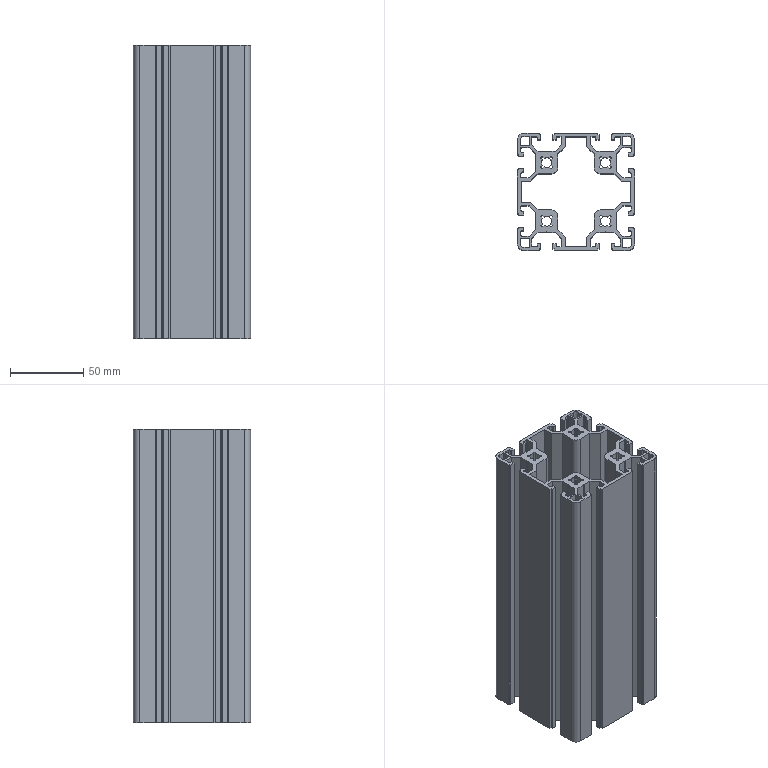Part | NX | features BREP 1 | 1 solid | 358 faces | box 80 x 80 x 200 mm | volume 343573 mm3 | plane 266 | cylinder 92 | commonest cylinder face diameters 0.6 x32 1 x16 2 x16 6.8 x16 5 x4 8 x4